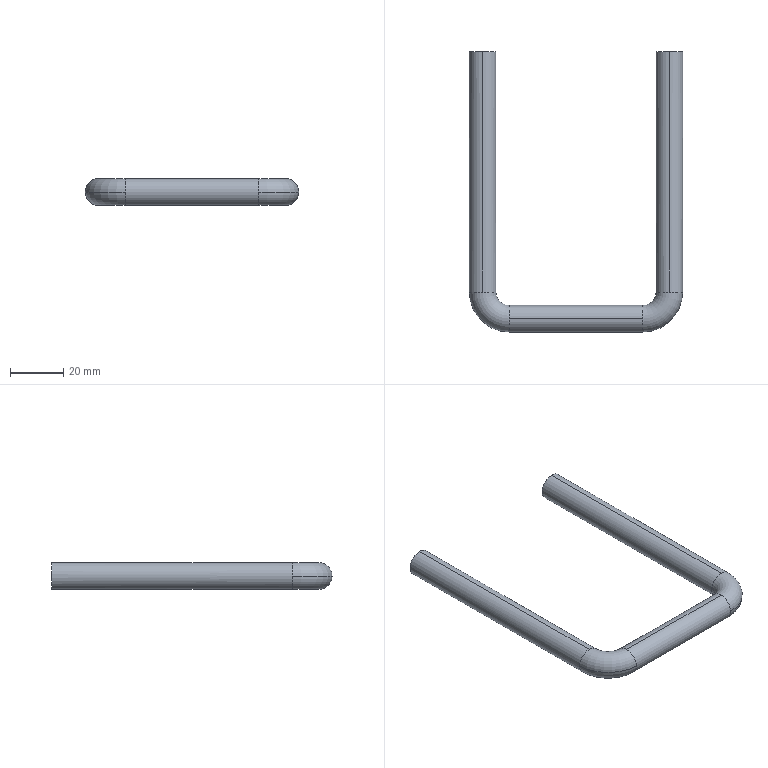Part | SolidWorks | features Sweep 1 | 1 solid | 12 faces | box 80 x 105 x 10 mm | volume 20532 mm3 | cylinder 6 | torus 4 | plane 2 | commonest cylinder face diameters 10 x6
STEP:
#1=CARTESIAN_POINT('',(-25.,0.,-5.));
#2=VERTEX_POINT('',#1);
#3=CARTESIAN_POINT('',(-25.,-5.,0.));
#4=VERTEX_POINT('',#3);
#5=CARTESIAN_POINT('',(-25.,0.,0.));
#6=DIRECTION('',(-1.,0.,0.));
#7=DIRECTION('',(0.,0.,-1.));
#8=AXIS2_PLACEMENT_3D('',#5,#6,#7);
#9=CIRCLE('',#8,5.);
#10=EDGE_CURVE('',#2,#4,#9,.T.);
#11=ORIENTED_EDGE('',*,*,#10,.T.);
#12=CARTESIAN_POINT('',(-40.,10.,0.));
#13=VERTEX_POINT('',#12);
#14=CARTESIAN_POINT('',(-25.,10.,0.));
#15=DIRECTION('',(0.,0.,-1.));
#16=DIRECTION('',(-1.,0.,0.));
#17=AXIS2_PLACEMENT_3D('',#14,#15,#16);
#18=CIRCLE('',#17,15.);
#19=EDGE_CURVE('',#4,#13,#18,.T.);
#20=ORIENTED_EDGE('',*,*,#19,.T.);
#21=CARTESIAN_POINT('',(-35.,10.,-5.));
#22=VERTEX_POINT('',#21);
#23=CARTESIAN_POINT('',(-35.,10.,0.));
#24=DIRECTION('',(0.,1.,0.));
#25=DIRECTION('',(0.,0.,-1.));
#26=AXIS2_PLACEMENT_3D('',#23,#24,#25);
#27=CIRCLE('',#26,5.);
#28=EDGE_CURVE('',#22,#13,#27,.T.);
#29=ORIENTED_EDGE('',*,*,#28,.F.);
#30=CARTESIAN_POINT('',(-30.,10.,0.));
#31=VERTEX_POINT('',#30);
#32=CARTESIAN_POINT('',(-35.,10.,0.));
#33=DIRECTION('',(0.,1.,0.));
#34=DIRECTION('',(0.,0.,-1.));
#35=AXIS2_PLACEMENT_3D('',#32,#33,#34);
#36=CIRCLE('',#35,5.);
#37=EDGE_CURVE('',#31,#22,#36,.T.);
#38=ORIENTED_EDGE('',*,*,#37,.F.);
#39=CARTESIAN_POINT('',(-25.,5.,0.));
#40=VERTEX_POINT('',#39);
#41=CARTESIAN_POINT('',(-25.,10.,0.));
#42=DIRECTION('',(0.,0.,-1.));
#43=DIRECTION('',(-1.,0.,0.));
#44=AXIS2_PLACEMENT_3D('',#41,#42,#43);
#45=CIRCLE('',#44,5.);
#46=EDGE_CURVE('',#40,#31,#45,.T.);
#47=ORIENTED_EDGE('',*,*,#46,.F.);
#48=CARTESIAN_POINT('',(-25.,0.,0.));
#49=DIRECTION('',(-1.,0.,0.));
#50=DIRECTION('',(0.,0.,-1.));
#51=AXIS2_PLACEMENT_3D('',#48,#49,#50);
#52=CIRCLE('',#51,5.);
#53=EDGE_CURVE('',#40,#2,#52,.T.);
#54=ORIENTED_EDGE('',*,*,#53,.T.);
#55=EDGE_LOOP('',(#11,#20,#29,#38,#47,#54));
#56=FACE_OUTER_BOUND('',#55,.T.);
#57=CARTESIAN_POINT('',(-25.,10.,0.));
#58=DIRECTION('',(0.,0.,-1.));
#59=DIRECTION('',(-1.,0.,0.));
#60=AXIS2_PLACEMENT_3D('',#57,#58,#59);
#61=TOROIDAL_SURFACE('',#60,10.,5.);
#62=ADVANCED_FACE('',(#56),#61,.T.);
#63=CARTESIAN_POINT('',(35.,10.,-5.));
#64=VERTEX_POINT('',#63);
#65=CARTESIAN_POINT('',(40.,10.,0.));
#66=VERTEX_POINT('',#65);
#67=CARTESIAN_POINT('',(35.,10.,0.));
#68=DIRECTION('',(0.,-1.,0.));
#69=DIRECTION('',(0.,0.,-1.));
#70=AXIS2_PLACEMENT_3D('',#67,#68,#69);
#71=CIRCLE('',#70,5.);
#72=EDGE_CURVE('',#64,#66,#71,.T.);
#73=ORIENTED_EDGE('',*,*,#72,.T.);
#74=CARTESIAN_POINT('',(25.,-5.,0.));
#75=VERTEX_POINT('',#74);
#76=CARTESIAN_POINT('',(25.,10.,0.));
#77=DIRECTION('',(0.,0.,-1.));
#78=DIRECTION('',(-1.,0.,0.));
#79=AXIS2_PLACEMENT_3D('',#76,#77,#78);
#80=CIRCLE('',#79,15.);
#81=EDGE_CURVE('',#66,#75,#80,.T.);
#82=ORIENTED_EDGE('',*,*,#81,.T.);
#83=CARTESIAN_POINT('',(25.,0.,-5.));
#84=VERTEX_POINT('',#83);
#85=CARTESIAN_POINT('',(25.,0.,0.));
#86=DIRECTION('',(-1.,0.,0.));
#87=DIRECTION('',(0.,0.,-1.));
#88=AXIS2_PLACEMENT_3D('',#85,#86,#87);
#89=CIRCLE('',#88,5.);
#90=EDGE_CURVE('',#84,#75,#89,.T.);
#91=ORIENTED_EDGE('',*,*,#90,.F.);
#92=CARTESIAN_POINT('',(25.,5.,0.));
#93=VERTEX_POINT('',#92);
#94=CARTESIAN_POINT('',(25.,0.,0.));
#95=DIRECTION('',(-1.,0.,0.));
#96=DIRECTION('',(0.,0.,-1.));
#97=AXIS2_PLACEMENT_3D('',#94,#95,#96);
#98=CIRCLE('',#97,5.);
#99=EDGE_CURVE('',#93,#84,#98,.T.);
#100=ORIENTED_EDGE('',*,*,#99,.F.);
#101=CARTESIAN_POINT('',(30.,10.,0.));
#102=VERTEX_POINT('',#101);
#103=CARTESIAN_POINT('',(25.,10.,0.));
#104=DIRECTION('',(0.,0.,-1.));
#105=DIRECTION('',(-1.,0.,0.));
#106=AXIS2_PLACEMENT_3D('',#103,#104,#105);
#107=CIRCLE('',#106,5.);
#108=EDGE_CURVE('',#102,#93,#107,.T.);
#109=ORIENTED_EDGE('',*,*,#108,.F.);
#110=CARTESIAN_POINT('',(35.,10.,0.));
#111=DIRECTION('',(0.,-1.,0.));
#112=DIRECTION('',(0.,0.,-1.));
#113=AXIS2_PLACEMENT_3D('',#110,#111,#112);
#114=CIRCLE('',#113,5.);
#115=EDGE_CURVE('',#102,#64,#114,.T.);
#116=ORIENTED_EDGE('',*,*,#115,.T.);
#117=EDGE_LOOP('',(#73,#82,#91,#100,#109,#116));
#118=FACE_OUTER_BOUND('',#117,.T.);
#119=CARTESIAN_POINT('',(25.,10.,0.));
#120=DIRECTION('',(0.,0.,-1.));
#121=DIRECTION('',(-1.,0.,0.));
#122=AXIS2_PLACEMENT_3D('',#119,#120,#121);
#123=TOROIDAL_SURFACE('',#122,10.,5.);
#124=ADVANCED_FACE('',(#118),#123,.T.);
#125=CARTESIAN_POINT('',(-35.,10.,5.));
#126=VERTEX_POINT('',#125);
#127=CARTESIAN_POINT('',(-35.,10.,0.));
#128=DIRECTION('',(0.,1.,0.));
#129=DIRECTION('',(0.,0.,-1.));
#130=AXIS2_PLACEMENT_3D('',#127,#128,#129);
#131=CIRCLE('',#130,5.);
#132=EDGE_CURVE('',#126,#31,#131,.T.);
#133=ORIENTED_EDGE('',*,*,#132,.T.);
#134=ORIENTED_EDGE('',*,*,#37,.T.);
#135=CARTESIAN_POINT('',(-35.,100.,-5.));
#136=VERTEX_POINT('',#135);
#137=CARTESIAN_POINT('',(-35.,10.,-5.));
#138=DIRECTION('',(0.,1.,0.));
#139=VECTOR('',#138,1000.);
#140=LINE('',#137,#139);
#141=EDGE_CURVE('',#22,#136,#140,.T.);
#142=ORIENTED_EDGE('',*,*,#141,.T.);
#143=CARTESIAN_POINT('',(-35.,100.,5.));
#144=VERTEX_POINT('',#143);
#145=CARTESIAN_POINT('',(-35.,100.,0.));
#146=DIRECTION('',(0.,1.,0.));
#147=DIRECTION('',(0.,0.,-1.));
#148=AXIS2_PLACEMENT_3D('',#145,#146,#147);
#149=CIRCLE('',#148,5.);
#150=EDGE_CURVE('',#144,#136,#149,.T.);
#151=ORIENTED_EDGE('',*,*,#150,.F.);
#152=CARTESIAN_POINT('',(-35.,10.,5.));
#153=DIRECTION('',(0.,1.,0.));
#154=VECTOR('',#153,1000.);
#155=LINE('',#152,#154);
#156=EDGE_CURVE('',#126,#144,#155,.T.);
#157=ORIENTED_EDGE('',*,*,#156,.F.);
#158=EDGE_LOOP('',(#133,#134,#142,#151,#157));
#159=FACE_OUTER_BOUND('',#158,.T.);
#160=CARTESIAN_POINT('',(-35.,10.,0.));
#161=DIRECTION('',(0.,1.,0.));
#162=DIRECTION('',(0.,0.,1.));
#163=AXIS2_PLACEMENT_3D('',#160,#161,#162);
#164=CYLINDRICAL_SURFACE('',#163,5.);
#165=ADVANCED_FACE('',(#159),#164,.T.);
#166=CARTESIAN_POINT('',(25.,0.,5.));
#167=VERTEX_POINT('',#166);
#168=CARTESIAN_POINT('',(25.,0.,0.));
#169=DIRECTION('',(-1.,0.,0.));
#170=DIRECTION('',(0.,0.,-1.));
#171=AXIS2_PLACEMENT_3D('',#168,#169,#170);
#172=CIRCLE('',#171,5.);
#173=EDGE_CURVE('',#167,#93,#172,.T.);
#174=ORIENTED_EDGE('',*,*,#173,.T.);
#175=ORIENTED_EDGE('',*,*,#99,.T.);
#176=CARTESIAN_POINT('',(25.,0.,-5.));
#177=DIRECTION('',(-1.,0.,0.));
#178=VECTOR('',#177,1000.);
#179=LINE('',#176,#178);
#180=EDGE_CURVE('',#84,#2,#179,.T.);
#181=ORIENTED_EDGE('',*,*,#180,.T.);
#182=ORIENTED_EDGE('',*,*,#53,.F.);
#183=CARTESIAN_POINT('',(-25.,0.,5.));
#184=VERTEX_POINT('',#183);
#185=CARTESIAN_POINT('',(-25.,0.,0.));
#186=DIRECTION('',(-1.,0.,0.));
#187=DIRECTION('',(0.,0.,-1.));
#188=AXIS2_PLACEMENT_3D('',#185,#186,#187);
#189=CIRCLE('',#188,5.);
#190=EDGE_CURVE('',#184,#40,#189,.T.);
#191=ORIENTED_EDGE('',*,*,#190,.F.);
#192=CARTESIAN_POINT('',(25.,0.,5.));
#193=DIRECTION('',(-1.,0.,0.));
#194=VECTOR('',#193,1000.);
#195=LINE('',#192,#194);
#196=EDGE_CURVE('',#167,#184,#195,.T.);
#197=ORIENTED_EDGE('',*,*,#196,.F.);
#198=EDGE_LOOP('',(#174,#175,#181,#182,#191,#197));
#199=FACE_OUTER_BOUND('',#198,.T.);
#200=CARTESIAN_POINT('',(25.,0.,0.));
#201=DIRECTION('',(-1.,0.,0.));
#202=DIRECTION('',(0.,0.,1.));
#203=AXIS2_PLACEMENT_3D('',#200,#201,#202);
#204=CYLINDRICAL_SURFACE('',#203,5.);
#205=ADVANCED_FACE('',(#199),#204,.T.);
#206=CARTESIAN_POINT('',(35.,100.,-5.));
#207=VERTEX_POINT('',#206);
#208=CARTESIAN_POINT('',(35.,100.,5.));
#209=VERTEX_POINT('',#208);
#210=CARTESIAN_POINT('',(35.,100.,0.));
#211=DIRECTION('',(0.,-1.,0.));
#212=DIRECTION('',(0.,0.,-1.));
#213=AXIS2_PLACEMENT_3D('',#210,#211,#212);
#214=CIRCLE('',#213,5.);
#215=EDGE_CURVE('',#207,#209,#214,.T.);
#216=ORIENTED_EDGE('',*,*,#215,.T.);
#217=CARTESIAN_POINT('',(35.,10.,5.));
#218=VERTEX_POINT('',#217);
#219=CARTESIAN_POINT('',(35.,100.,5.));
#220=DIRECTION('',(0.,-1.,0.));
#221=VECTOR('',#220,1000.);
#222=LINE('',#219,#221);
#223=EDGE_CURVE('',#209,#218,#222,.T.);
#224=ORIENTED_EDGE('',*,*,#223,.T.);
#225=CARTESIAN_POINT('',(35.,10.,0.));
#226=DIRECTION('',(0.,-1.,0.));
#227=DIRECTION('',(0.,0.,-1.));
#228=AXIS2_PLACEMENT_3D('',#225,#226,#227);
#229=CIRCLE('',#228,5.);
#230=EDGE_CURVE('',#66,#218,#229,.T.);
#231=ORIENTED_EDGE('',*,*,#230,.F.);
#232=ORIENTED_EDGE('',*,*,#72,.F.);
#233=CARTESIAN_POINT('',(35.,100.,-5.));
#234=DIRECTION('',(0.,-1.,0.));
#235=VECTOR('',#234,1000.);
#236=LINE('',#233,#235);
#237=EDGE_CURVE('',#207,#64,#236,.T.);
#238=ORIENTED_EDGE('',*,*,#237,.F.);
#239=EDGE_LOOP('',(#216,#224,#231,#232,#238));
#240=FACE_OUTER_BOUND('',#239,.T.);
#241=CARTESIAN_POINT('',(35.,100.,0.));
#242=DIRECTION('',(0.,-1.,0.));
#243=DIRECTION('',(0.,0.,-1.));
#244=AXIS2_PLACEMENT_3D('',#241,#242,#243);
#245=CYLINDRICAL_SURFACE('',#244,5.);
#246=ADVANCED_FACE('',(#240),#245,.T.);
#247=ORIENTED_EDGE('',*,*,#141,.F.);
#248=ORIENTED_EDGE('',*,*,#28,.T.);
#249=CARTESIAN_POINT('',(-35.,10.,0.));
#250=DIRECTION('',(0.,1.,0.));
#251=DIRECTION('',(0.,0.,-1.));
#252=AXIS2_PLACEMENT_3D('',#249,#250,#251);
#253=CIRCLE('',#252,5.);
#254=EDGE_CURVE('',#13,#126,#253,.T.);
#255=ORIENTED_EDGE('',*,*,#254,.T.);
#256=ORIENTED_EDGE('',*,*,#156,.T.);
#257=CARTESIAN_POINT('',(-35.,100.,0.));
#258=DIRECTION('',(0.,1.,0.));
#259=DIRECTION('',(0.,0.,-1.));
#260=AXIS2_PLACEMENT_3D('',#257,#258,#259);
#261=CIRCLE('',#260,5.);
#262=EDGE_CURVE('',#136,#144,#261,.T.);
#263=ORIENTED_EDGE('',*,*,#262,.F.);
#264=EDGE_LOOP('',(#247,#248,#255,#256,#263));
#265=FACE_OUTER_BOUND('',#264,.T.);
#266=CARTESIAN_POINT('',(-35.,10.,0.));
#267=DIRECTION('',(0.,1.,0.));
#268=DIRECTION('',(0.,0.,1.));
#269=AXIS2_PLACEMENT_3D('',#266,#267,#268);
#270=CYLINDRICAL_SURFACE('',#269,5.);
#271=ADVANCED_FACE('',(#265),#270,.T.);
#272=ORIENTED_EDGE('',*,*,#19,.F.);
#273=CARTESIAN_POINT('',(-25.,0.,0.));
#274=DIRECTION('',(-1.,0.,0.));
#275=DIRECTION('',(0.,0.,-1.));
#276=AXIS2_PLACEMENT_3D('',#273,#274,#275);
#277=CIRCLE('',#276,5.);
#278=EDGE_CURVE('',#4,#184,#277,.T.);
#279=ORIENTED_EDGE('',*,*,#278,.T.);
#280=ORIENTED_EDGE('',*,*,#190,.T.);
#281=ORIENTED_EDGE('',*,*,#46,.T.);
#282=ORIENTED_EDGE('',*,*,#132,.F.);
#283=ORIENTED_EDGE('',*,*,#254,.F.);
#284=EDGE_LOOP('',(#272,#279,#280,#281,#282,#283));
#285=FACE_OUTER_BOUND('',#284,.T.);
#286=CARTESIAN_POINT('',(-25.,10.,0.));
#287=DIRECTION('',(0.,0.,-1.));
#288=DIRECTION('',(-1.,0.,0.));
#289=AXIS2_PLACEMENT_3D('',#286,#287,#288);
#290=TOROIDAL_SURFACE('',#289,10.,5.);
#291=ADVANCED_FACE('',(#285),#290,.T.);
#292=ORIENTED_EDGE('',*,*,#180,.F.);
#293=ORIENTED_EDGE('',*,*,#90,.T.);
#294=CARTESIAN_POINT('',(25.,0.,0.));
#295=DIRECTION('',(-1.,0.,0.));
#296=DIRECTION('',(0.,0.,-1.));
#297=AXIS2_PLACEMENT_3D('',#294,#295,#296);
#298=CIRCLE('',#297,5.);
#299=EDGE_CURVE('',#75,#167,#298,.T.);
#300=ORIENTED_EDGE('',*,*,#299,.T.);
#301=ORIENTED_EDGE('',*,*,#196,.T.);
#302=ORIENTED_EDGE('',*,*,#278,.F.);
#303=ORIENTED_EDGE('',*,*,#10,.F.);
#304=EDGE_LOOP('',(#292,#293,#300,#301,#302,#303));
#305=FACE_OUTER_BOUND('',#304,.T.);
#306=CARTESIAN_POINT('',(25.,0.,0.));
#307=DIRECTION('',(-1.,0.,0.));
#308=DIRECTION('',(0.,0.,1.));
#309=AXIS2_PLACEMENT_3D('',#306,#307,#308);
#310=CYLINDRICAL_SURFACE('',#309,5.);
#311=ADVANCED_FACE('',(#305),#310,.T.);
#312=ORIENTED_EDGE('',*,*,#81,.F.);
#313=ORIENTED_EDGE('',*,*,#230,.T.);
#314=CARTESIAN_POINT('',(35.,10.,0.));
#315=DIRECTION('',(0.,-1.,0.));
#316=DIRECTION('',(0.,0.,-1.));
#317=AXIS2_PLACEMENT_3D('',#314,#315,#316);
#318=CIRCLE('',#317,5.);
#319=EDGE_CURVE('',#218,#102,#318,.T.);
#320=ORIENTED_EDGE('',*,*,#319,.T.);
#321=ORIENTED_EDGE('',*,*,#108,.T.);
#322=ORIENTED_EDGE('',*,*,#173,.F.);
#323=ORIENTED_EDGE('',*,*,#299,.F.);
#324=EDGE_LOOP('',(#312,#313,#320,#321,#322,#323));
#325=FACE_OUTER_BOUND('',#324,.T.);
#326=CARTESIAN_POINT('',(25.,10.,0.));
#327=DIRECTION('',(0.,0.,-1.));
#328=DIRECTION('',(-1.,0.,0.));
#329=AXIS2_PLACEMENT_3D('',#326,#327,#328);
#330=TOROIDAL_SURFACE('',#329,10.,5.);
#331=ADVANCED_FACE('',(#325),#330,.T.);
#332=ORIENTED_EDGE('',*,*,#223,.F.);
#333=CARTESIAN_POINT('',(35.,100.,0.));
#334=DIRECTION('',(0.,-1.,0.));
#335=DIRECTION('',(0.,0.,-1.));
#336=AXIS2_PLACEMENT_3D('',#333,#334,#335);
#337=CIRCLE('',#336,5.);
#338=EDGE_CURVE('',#209,#207,#337,.T.);
#339=ORIENTED_EDGE('',*,*,#338,.T.);
#340=ORIENTED_EDGE('',*,*,#237,.T.);
#341=ORIENTED_EDGE('',*,*,#115,.F.);
#342=ORIENTED_EDGE('',*,*,#319,.F.);
#343=EDGE_LOOP('',(#332,#339,#340,#341,#342));
#344=FACE_OUTER_BOUND('',#343,.T.);
#345=CARTESIAN_POINT('',(35.,100.,0.));
#346=DIRECTION('',(0.,-1.,0.));
#347=DIRECTION('',(0.,0.,-1.));
#348=AXIS2_PLACEMENT_3D('',#345,#346,#347);
#349=CYLINDRICAL_SURFACE('',#348,5.);
#350=ADVANCED_FACE('',(#344),#349,.T.);
#351=ORIENTED_EDGE('',*,*,#150,.T.);
#352=ORIENTED_EDGE('',*,*,#262,.T.);
#353=EDGE_LOOP('',(#351,#352));
#354=FACE_OUTER_BOUND('',#353,.T.);
#355=CARTESIAN_POINT('',(-35.,100.,0.));
#356=DIRECTION('',(0.,1.,0.));
#357=DIRECTION('',(0.,0.,-1.));
#358=AXIS2_PLACEMENT_3D('',#355,#356,#357);
#359=PLANE('',#358);
#360=ADVANCED_FACE('',(#354),#359,.T.);
#361=ORIENTED_EDGE('',*,*,#215,.F.);
#362=ORIENTED_EDGE('',*,*,#338,.F.);
#363=EDGE_LOOP('',(#361,#362));
#364=FACE_OUTER_BOUND('',#363,.T.);
#365=CARTESIAN_POINT('',(35.,100.,0.));
#366=DIRECTION('',(0.,-1.,0.));
#367=DIRECTION('',(0.,0.,-1.));
#368=AXIS2_PLACEMENT_3D('',#365,#366,#367);
#369=PLANE('',#368);
#370=ADVANCED_FACE('',(#364),#369,.F.);
#371=CLOSED_SHELL('',(#62,#124,#165,#205,#246,#271,#291,#311,#331,#350,#360,#370));
#372=MANIFOLD_SOLID_BREP('',#371);
#373=CARTESIAN_POINT('',(0.,0.,0.));
#374=DIRECTION('',(0.,0.,1.));
#375=DIRECTION('',(1.,0.,0.));
#376=AXIS2_PLACEMENT_3D('',#373,#374,#375);
#377=(LENGTH_UNIT()NAMED_UNIT(*)SI_UNIT(.MILLI.,.METRE.));
#378=UNCERTAINTY_MEASURE_WITH_UNIT(LENGTH_MEASURE(0.00001),#377,'','');
#379=(NAMED_UNIT(*)PLANE_ANGLE_UNIT()SI_UNIT($,.RADIAN.));
#380=(NAMED_UNIT(*)SI_UNIT($,.STERADIAN.)SOLID_ANGLE_UNIT());
#381=(GEOMETRIC_REPRESENTATION_CONTEXT(3)GLOBAL_UNCERTAINTY_ASSIGNED_CONTEXT((#378))GLOBAL_UNIT_ASSIGNED_CONTEXT((#377,#379,#380))REPRESENTATION_CONTEXT('',''));
#382=ADVANCED_BREP_SHAPE_REPRESENTATION('',(#372,#376),#381);